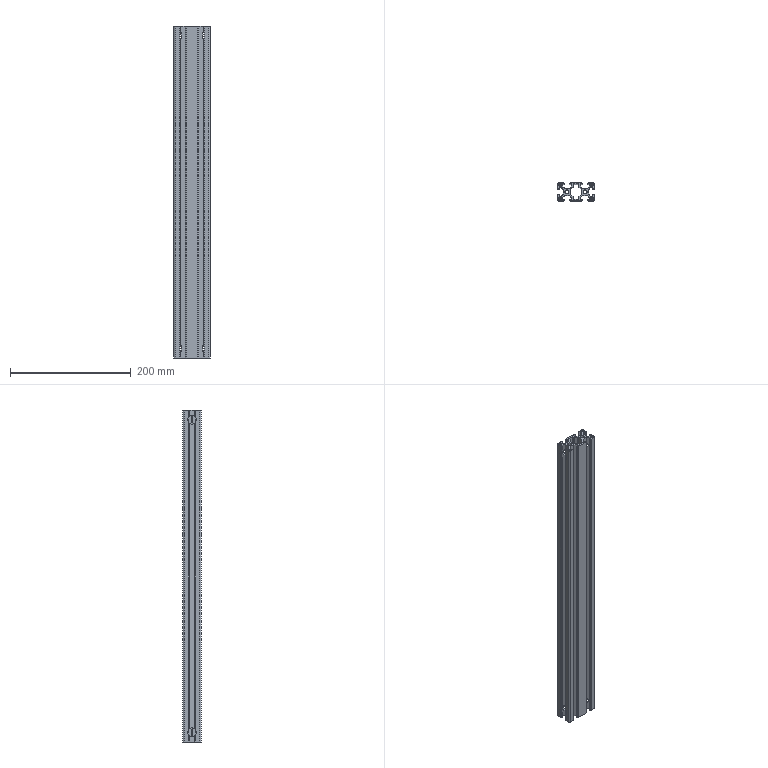Part | NX | features BREP 1 | 1 solid | 348 faces | box 60 x 30 x 550 mm | volume 326573 mm3 | cylinder 188 | plane 160 | commonest cylinder face diameters 0.6 x132 2 x28 15 x20 4 x4 6.8 x4